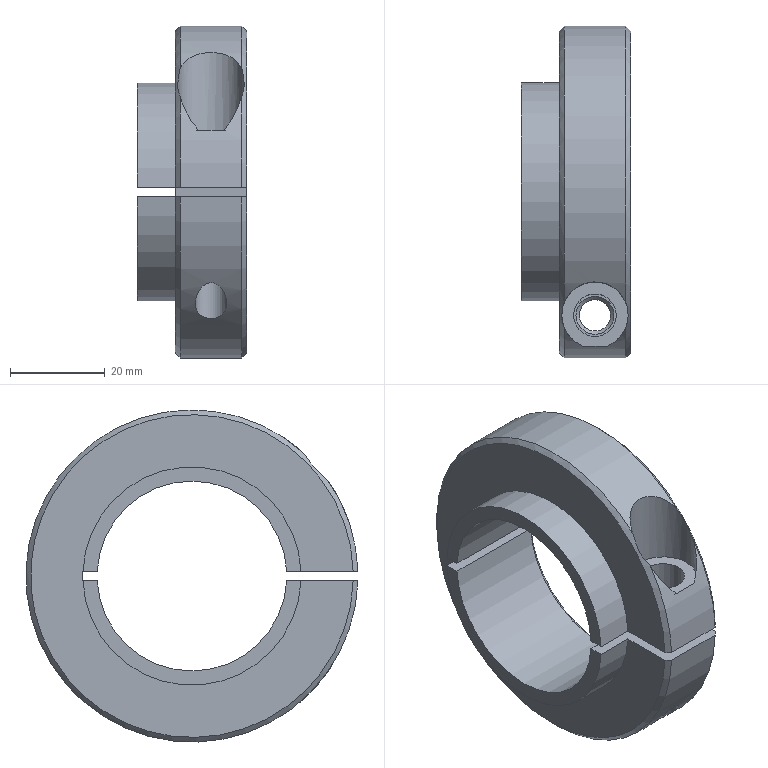Part | NX | features 1_52 2 | 1 solid | 24 faces | box 23 x 69.986 x 70 mm | volume 38156 mm3 | plane 10 | cylinder 9 | cone 5 | commonest cylinder face diameters 40 x2 46 x2 70 x2 6.647 x1 9 x1 14 x1
STEP:
#1=CARTESIAN_POINT('',(-138.5,-99.025,-821.129));
#2=VERTEX_POINT('',#1);
#3=CARTESIAN_POINT('',(-138.5,-138.975,-821.129));
#4=VERTEX_POINT('',#3);
#5=CARTESIAN_POINT('',(-138.5,-119.,-820.129));
#6=DIRECTION('',(-1.,0.,0.));
#7=DIRECTION('',(0.,0.,-1.));
#8=AXIS2_PLACEMENT_3D('',#5,#6,#7);
#9=CIRCLE('',#8,20.);
#10=EDGE_CURVE('',#2,#4,#9,.T.);
#11=ORIENTED_EDGE('',*,*,#10,.T.);
#12=CARTESIAN_POINT('',(-137.5,-139.976,-821.129));
#13=VERTEX_POINT('',#12);
#14=CARTESIAN_POINT('',(-137.5,-139.976,-821.129));
#15=CARTESIAN_POINT('',(-137.833,-139.642,-821.129));
#16=CARTESIAN_POINT('',(-138.167,-139.309,-821.129));
#17=CARTESIAN_POINT('',(-138.5,-138.975,-821.129));
#18=B_SPLINE_CURVE_WITH_KNOTS('',3,(#14,#15,#16,#17),.UNSPECIFIED.,.F.,.F.,(4,4),(0.,1.),.UNSPECIFIED.);
#19=EDGE_CURVE('',#4,#13,#18,.F.);
#20=ORIENTED_EDGE('',*,*,#19,.T.);
#21=CARTESIAN_POINT('',(-137.5,-98.024,-821.129));
#22=VERTEX_POINT('',#21);
#23=CARTESIAN_POINT('',(-137.5,-119.,-820.129));
#24=DIRECTION('',(-1.,0.,0.));
#25=DIRECTION('',(0.,0.,-1.));
#26=AXIS2_PLACEMENT_3D('',#23,#24,#25);
#27=CIRCLE('',#26,21.);
#28=EDGE_CURVE('',#22,#13,#27,.T.);
#29=ORIENTED_EDGE('',*,*,#28,.F.);
#30=CARTESIAN_POINT('',(-138.5,-99.025,-821.129));
#31=CARTESIAN_POINT('',(-138.167,-98.691,-821.129));
#32=CARTESIAN_POINT('',(-137.833,-98.358,-821.129));
#33=CARTESIAN_POINT('',(-137.5,-98.024,-821.129));
#34=B_SPLINE_CURVE_WITH_KNOTS('',3,(#30,#31,#32,#33),.UNSPECIFIED.,.F.,.F.,(4,4),(0.,1.),.UNSPECIFIED.);
#35=EDGE_CURVE('',#22,#2,#34,.F.);
#36=ORIENTED_EDGE('',*,*,#35,.T.);
#37=EDGE_LOOP('',(#11,#20,#29,#36));
#38=FACE_BOUND('',#37,.T.);
#39=CARTESIAN_POINT('',(-138.586,-119.,-820.129));
#40=DIRECTION('',(1.,0.,0.));
#41=DIRECTION('',(0.,0.,-1.));
#42=AXIS2_PLACEMENT_3D('',#39,#40,#41);
#43=CONICAL_SURFACE('',#42,19.914,0.7854);
#44=ADVANCED_FACE('',(#38),#43,.F.);
#45=CARTESIAN_POINT('',(-149.5,-145.,-819.129));
#46=VERTEX_POINT('',#45);
#47=CARTESIAN_POINT('',(-145.,-145.,-819.129));
#48=DIRECTION('',(0.,0.,1.));
#49=DIRECTION('',(-1.,0.,0.));
#50=AXIS2_PLACEMENT_3D('',#47,#48,#49);
#51=CIRCLE('',#50,4.5);
#52=EDGE_CURVE('',#46,#46,#51,.T.);
#53=ORIENTED_EDGE('',*,*,#52,.F.);
#54=EDGE_LOOP('',(#53));
#55=FACE_BOUND('',#54,.T.);
#56=CARTESIAN_POINT('',(-140.5,-145.,-807.129));
#57=VERTEX_POINT('',#56);
#58=CARTESIAN_POINT('',(-145.,-145.,-807.129));
#59=DIRECTION('',(0.,0.,-1.));
#60=DIRECTION('',(1.,0.,0.));
#61=AXIS2_PLACEMENT_3D('',#58,#59,#60);
#62=CIRCLE('',#61,4.5);
#63=EDGE_CURVE('',#57,#57,#62,.T.);
#64=ORIENTED_EDGE('',*,*,#63,.F.);
#65=EDGE_LOOP('',(#64));
#66=FACE_BOUND('',#65,.T.);
#67=CARTESIAN_POINT('',(-145.,-145.,-813.629));
#68=DIRECTION('',(0.,0.,1.));
#69=DIRECTION('',(1.,0.,0.));
#70=AXIS2_PLACEMENT_3D('',#67,#68,#69);
#71=CYLINDRICAL_SURFACE('',#70,4.5);
#72=ADVANCED_FACE('',(#55,#66),#71,.F.);
#73=CARTESIAN_POINT('',(-141.677,-145.,-821.806));
#74=VERTEX_POINT('',#73);
#75=CARTESIAN_POINT('',(-145.,-145.,-821.806));
#76=DIRECTION('',(0.,0.,-1.));
#77=DIRECTION('',(1.,0.,0.));
#78=AXIS2_PLACEMENT_3D('',#75,#76,#77);
#79=CIRCLE('',#78,3.323);
#80=EDGE_CURVE('',#74,#74,#79,.T.);
#81=ORIENTED_EDGE('',*,*,#80,.T.);
#82=EDGE_LOOP('',(#81));
#83=FACE_BOUND('',#82,.T.);
#84=CARTESIAN_POINT('',(-149.,-145.,-821.129));
#85=VERTEX_POINT('',#84);
#86=CARTESIAN_POINT('',(-145.,-145.,-821.129));
#87=DIRECTION('',(0.,0.,-1.));
#88=DIRECTION('',(-1.,0.,0.));
#89=AXIS2_PLACEMENT_3D('',#86,#87,#88);
#90=CIRCLE('',#89,4.);
#91=EDGE_CURVE('',#85,#85,#90,.T.);
#92=ORIENTED_EDGE('',*,*,#91,.F.);
#93=EDGE_LOOP('',(#92));
#94=FACE_BOUND('',#93,.T.);
#95=CARTESIAN_POINT('',(-145.,-145.,-821.892));
#96=DIRECTION('',(0.,0.,1.));
#97=DIRECTION('',(1.,0.,0.));
#98=AXIS2_PLACEMENT_3D('',#95,#96,#97);
#99=CONICAL_SURFACE('',#98,3.237,0.7854);
#100=ADVANCED_FACE('',(#83,#94),#99,.F.);
#101=CARTESIAN_POINT('',(-141.677,-145.,-843.56));
#102=VERTEX_POINT('',#101);
#103=CARTESIAN_POINT('',(-148.323,-145.,-843.56));
#104=VERTEX_POINT('',#103);
#105=CARTESIAN_POINT('',(-148.323,-145.,-843.56));
#106=CARTESIAN_POINT('',(-148.323,-145.388,-843.13));
#107=CARTESIAN_POINT('',(-148.191,-146.141,-842.25));
#108=CARTESIAN_POINT('',(-147.617,-147.152,-840.945));
#109=CARTESIAN_POINT('',(-146.673,-147.999,-839.739));
#110=CARTESIAN_POINT('',(-145.,-148.486,-838.987));
#111=CARTESIAN_POINT('',(-143.327,-147.999,-839.739));
#112=CARTESIAN_POINT('',(-142.383,-147.152,-840.945));
#113=CARTESIAN_POINT('',(-141.809,-146.141,-842.25));
#114=CARTESIAN_POINT('',(-141.677,-145.388,-843.13));
#115=CARTESIAN_POINT('',(-141.677,-145.,-843.56));
#116=B_SPLINE_CURVE_WITH_KNOTS('',3,(#105,#106,#107,#108,#109,#110,#111,#112,#113,#114,#115),.UNSPECIFIED.,.F.,.F.,(4,1,1,1,1,1,1,1,4),(0.,0.125,0.25,0.375,0.5,0.625,0.75,0.875,1.),.UNSPECIFIED.);
#117=EDGE_CURVE('',#102,#104,#116,.F.);
#118=ORIENTED_EDGE('',*,*,#117,.T.);
#119=CARTESIAN_POINT('',(-141.677,-145.,-843.56));
#120=CARTESIAN_POINT('',(-141.677,-144.295,-844.34));
#121=CARTESIAN_POINT('',(-142.002,-143.157,-845.485));
#122=CARTESIAN_POINT('',(-143.428,-141.943,-846.565));
#123=CARTESIAN_POINT('',(-145.,-141.543,-846.902));
#124=CARTESIAN_POINT('',(-146.572,-141.943,-846.565));
#125=CARTESIAN_POINT('',(-147.998,-143.157,-845.486));
#126=CARTESIAN_POINT('',(-148.323,-144.295,-844.34));
#127=CARTESIAN_POINT('',(-148.323,-145.,-843.56));
#128=B_SPLINE_CURVE_WITH_KNOTS('',3,(#119,#120,#121,#122,#123,#124,#125,#126,#127),.UNSPECIFIED.,.F.,.F.,(4,1,1,1,1,1,4),(0.,0.25,0.375,0.5,0.625,0.75,1.),.UNSPECIFIED.);
#129=EDGE_CURVE('',#104,#102,#128,.F.);
#130=ORIENTED_EDGE('',*,*,#129,.T.);
#131=EDGE_LOOP('',(#118,#130));
#132=FACE_BOUND('',#131,.T.);
#133=ORIENTED_EDGE('',*,*,#80,.F.);
#134=EDGE_LOOP('',(#133));
#135=FACE_BOUND('',#134,.T.);
#136=CARTESIAN_POINT('',(-145.,-145.,-840.968));
#137=DIRECTION('',(0.,0.,-1.));
#138=DIRECTION('',(-1.,0.,0.));
#139=AXIS2_PLACEMENT_3D('',#136,#137,#138);
#140=CYLINDRICAL_SURFACE('',#139,3.324);
#141=ADVANCED_FACE('',(#132,#135),#140,.F.);
#142=CARTESIAN_POINT('',(-151.5,-142.402,-794.103));
#143=VERTEX_POINT('',#142);
#144=CARTESIAN_POINT('',(-151.5,-153.986,-821.129));
#145=VERTEX_POINT('',#144);
#146=CARTESIAN_POINT('',(-151.5,-119.,-820.129));
#147=DIRECTION('',(-1.,0.,0.));
#148=DIRECTION('',(0.,-0.6686,0.7436));
#149=AXIS2_PLACEMENT_3D('',#146,#147,#148);
#150=CIRCLE('',#149,35.);
#151=EDGE_CURVE('',#143,#145,#150,.T.);
#152=ORIENTED_EDGE('',*,*,#151,.F.);
#153=CARTESIAN_POINT('',(-138.5,-142.402,-794.103));
#154=VERTEX_POINT('',#153);
#155=CARTESIAN_POINT('',(-138.5,-142.402,-794.103));
#156=CARTESIAN_POINT('',(-138.933,-141.315,-793.126));
#157=CARTESIAN_POINT('',(-140.459,-139.092,-791.412));
#158=CARTESIAN_POINT('',(-145.,-137.454,-790.398));
#159=CARTESIAN_POINT('',(-149.541,-139.092,-791.412));
#160=CARTESIAN_POINT('',(-151.068,-141.315,-793.126));
#161=CARTESIAN_POINT('',(-151.5,-142.402,-794.103));
#162=B_SPLINE_CURVE_WITH_KNOTS('',3,(#155,#156,#157,#158,#159,#160,#161),.UNSPECIFIED.,.F.,.F.,(4,1,1,1,4),(0.,0.25,0.5,0.75,1.),.UNSPECIFIED.);
#163=EDGE_CURVE('',#154,#143,#162,.T.);
#164=ORIENTED_EDGE('',*,*,#163,.F.);
#165=CARTESIAN_POINT('',(-138.5,-153.986,-821.129));
#166=VERTEX_POINT('',#165);
#167=CARTESIAN_POINT('',(-138.5,-119.,-820.129));
#168=DIRECTION('',(1.,0.,0.));
#169=DIRECTION('',(0.,0.,1.));
#170=AXIS2_PLACEMENT_3D('',#167,#168,#169);
#171=CIRCLE('',#170,35.);
#172=EDGE_CURVE('',#166,#154,#171,.T.);
#173=ORIENTED_EDGE('',*,*,#172,.F.);
#174=CARTESIAN_POINT('',(-138.5,-153.986,-821.129));
#175=DIRECTION('',(-1.,0.,0.));
#176=VECTOR('',#175,1000.);
#177=LINE('',#174,#176);
#178=EDGE_CURVE('',#166,#145,#177,.T.);
#179=ORIENTED_EDGE('',*,*,#178,.T.);
#180=EDGE_LOOP('',(#152,#164,#173,#179));
#181=FACE_BOUND('',#180,.T.);
#182=ORIENTED_EDGE('',*,*,#129,.F.);
#183=ORIENTED_EDGE('',*,*,#117,.F.);
#184=EDGE_LOOP('',(#182,#183));
#185=FACE_BOUND('',#184,.T.);
#186=CARTESIAN_POINT('',(-145.,-119.,-820.129));
#187=DIRECTION('',(1.,0.,0.));
#188=DIRECTION('',(0.,0.,-1.));
#189=AXIS2_PLACEMENT_3D('',#186,#187,#188);
#190=CYLINDRICAL_SURFACE('',#189,35.);
#191=ADVANCED_FACE('',(#181,#185),#190,.T.);
#192=ORIENTED_EDGE('',*,*,#63,.T.);
#193=EDGE_LOOP('',(#192));
#194=FACE_BOUND('',#193,.T.);
#195=CARTESIAN_POINT('',(-142.392,-151.496,-807.129));
#196=VERTEX_POINT('',#195);
#197=CARTESIAN_POINT('',(-147.608,-151.496,-807.129));
#198=VERTEX_POINT('',#197);
#199=CARTESIAN_POINT('',(-142.392,-151.496,-807.129));
#200=DIRECTION('',(-1.,0.,0.));
#201=VECTOR('',#200,1000.);
#202=LINE('',#199,#201);
#203=EDGE_CURVE('',#196,#198,#202,.T.);
#204=ORIENTED_EDGE('',*,*,#203,.F.);
#205=CARTESIAN_POINT('',(-145.,-145.,-807.129));
#206=DIRECTION('',(0.,0.,1.));
#207=DIRECTION('',(-1.,0.,0.));
#208=AXIS2_PLACEMENT_3D('',#205,#206,#207);
#209=CIRCLE('',#208,7.);
#210=EDGE_CURVE('',#196,#198,#209,.T.);
#211=ORIENTED_EDGE('',*,*,#210,.T.);
#212=EDGE_LOOP('',(#204,#211));
#213=FACE_BOUND('',#212,.T.);
#214=CARTESIAN_POINT('',(-145.,-150.75,-807.129));
#215=DIRECTION('',(0.,0.,-1.));
#216=DIRECTION('',(-1.,0.,0.));
#217=AXIS2_PLACEMENT_3D('',#214,#215,#216);
#218=PLANE('',#217);
#219=ADVANCED_FACE('',(#194,#213),#218,.F.);
#220=ORIENTED_EDGE('',*,*,#210,.F.);
#221=CARTESIAN_POINT('',(-138.5,-147.598,-799.951));
#222=VERTEX_POINT('',#221);
#223=CARTESIAN_POINT('',(-138.5,-147.598,-799.951));
#224=CARTESIAN_POINT('',(-138.843,-148.455,-801.166));
#225=CARTESIAN_POINT('',(-139.839,-149.967,-803.636));
#226=CARTESIAN_POINT('',(-141.357,-151.081,-806.087));
#227=CARTESIAN_POINT('',(-142.392,-151.496,-807.129));
#228=B_SPLINE_CURVE_WITH_KNOTS('',3,(#223,#224,#225,#226,#227),.UNSPECIFIED.,.F.,.F.,(4,1,4),(0.,0.5,1.),.UNSPECIFIED.);
#229=EDGE_CURVE('',#196,#222,#228,.F.);
#230=ORIENTED_EDGE('',*,*,#229,.T.);
#231=CARTESIAN_POINT('',(-138.,-145.,-797.452));
#232=VERTEX_POINT('',#231);
#233=CARTESIAN_POINT('',(-138.,-145.,-797.452));
#234=CARTESIAN_POINT('',(-138.,-145.806,-798.364));
#235=CARTESIAN_POINT('',(-138.124,-146.657,-799.264));
#236=CARTESIAN_POINT('',(-138.5,-147.598,-799.951));
#237=B_SPLINE_CURVE_WITH_KNOTS('',3,(#233,#234,#235,#236),.UNSPECIFIED.,.F.,.F.,(4,4),(0.,1.),.UNSPECIFIED.);
#238=EDGE_CURVE('',#222,#232,#237,.F.);
#239=ORIENTED_EDGE('',*,*,#238,.T.);
#240=CARTESIAN_POINT('',(-138.5,-142.402,-794.103));
#241=CARTESIAN_POINT('',(-138.182,-143.198,-795.243));
#242=CARTESIAN_POINT('',(-138.,-144.063,-796.376));
#243=CARTESIAN_POINT('',(-138.,-145.,-797.452));
#244=B_SPLINE_CURVE_WITH_KNOTS('',3,(#240,#241,#242,#243),.UNSPECIFIED.,.F.,.F.,(4,4),(0.,1.),.UNSPECIFIED.);
#245=EDGE_CURVE('',#232,#154,#244,.F.);
#246=ORIENTED_EDGE('',*,*,#245,.T.);
#247=ORIENTED_EDGE('',*,*,#163,.T.);
#248=CARTESIAN_POINT('',(-152.,-145.,-797.452));
#249=VERTEX_POINT('',#248);
#250=CARTESIAN_POINT('',(-152.,-145.,-797.452));
#251=CARTESIAN_POINT('',(-152.,-144.063,-796.376));
#252=CARTESIAN_POINT('',(-151.818,-143.198,-795.243));
#253=CARTESIAN_POINT('',(-151.5,-142.402,-794.103));
#254=B_SPLINE_CURVE_WITH_KNOTS('',3,(#250,#251,#252,#253),.UNSPECIFIED.,.F.,.F.,(4,4),(0.,1.),.UNSPECIFIED.);
#255=EDGE_CURVE('',#143,#249,#254,.F.);
#256=ORIENTED_EDGE('',*,*,#255,.T.);
#257=CARTESIAN_POINT('',(-151.5,-147.598,-799.951));
#258=VERTEX_POINT('',#257);
#259=CARTESIAN_POINT('',(-151.5,-147.598,-799.951));
#260=CARTESIAN_POINT('',(-151.876,-146.657,-799.264));
#261=CARTESIAN_POINT('',(-152.,-145.806,-798.363));
#262=CARTESIAN_POINT('',(-152.,-145.,-797.452));
#263=B_SPLINE_CURVE_WITH_KNOTS('',3,(#259,#260,#261,#262),.UNSPECIFIED.,.F.,.F.,(4,4),(0.,1.),.UNSPECIFIED.);
#264=EDGE_CURVE('',#249,#258,#263,.F.);
#265=ORIENTED_EDGE('',*,*,#264,.T.);
#266=CARTESIAN_POINT('',(-147.608,-151.496,-807.129));
#267=CARTESIAN_POINT('',(-148.643,-151.081,-806.087));
#268=CARTESIAN_POINT('',(-150.161,-149.967,-803.636));
#269=CARTESIAN_POINT('',(-151.157,-148.455,-801.166));
#270=CARTESIAN_POINT('',(-151.5,-147.598,-799.951));
#271=B_SPLINE_CURVE_WITH_KNOTS('',3,(#266,#267,#268,#269,#270),.UNSPECIFIED.,.F.,.F.,(4,1,4),(0.,0.5,1.),.UNSPECIFIED.);
#272=EDGE_CURVE('',#258,#198,#271,.F.);
#273=ORIENTED_EDGE('',*,*,#272,.T.);
#274=EDGE_LOOP('',(#220,#230,#239,#246,#247,#256,#265,#273));
#275=FACE_BOUND('',#274,.T.);
#276=CARTESIAN_POINT('',(-145.,-145.,-796.129));
#277=DIRECTION('',(0.,0.,1.));
#278=DIRECTION('',(1.,0.,0.));
#279=AXIS2_PLACEMENT_3D('',#276,#277,#278);
#280=CYLINDRICAL_SURFACE('',#279,7.);
#281=ADVANCED_FACE('',(#275),#280,.F.);
#282=CARTESIAN_POINT('',(-138.5,-153.986,-819.129));
#283=VERTEX_POINT('',#282);
#284=CARTESIAN_POINT('',(-138.5,-119.,-820.129));
#285=DIRECTION('',(1.,0.,0.));
#286=DIRECTION('',(0.,-0.8171,0.5765));
#287=AXIS2_PLACEMENT_3D('',#284,#285,#286);
#288=CIRCLE('',#287,35.);
#289=EDGE_CURVE('',#222,#283,#288,.T.);
#290=ORIENTED_EDGE('',*,*,#289,.F.);
#291=ORIENTED_EDGE('',*,*,#229,.F.);
#292=ORIENTED_EDGE('',*,*,#203,.T.);
#293=ORIENTED_EDGE('',*,*,#272,.F.);
#294=CARTESIAN_POINT('',(-151.5,-153.986,-819.129));
#295=VERTEX_POINT('',#294);
#296=CARTESIAN_POINT('',(-151.5,-119.,-820.129));
#297=DIRECTION('',(-1.,0.,0.));
#298=DIRECTION('',(0.,-0.9996,0.02857));
#299=AXIS2_PLACEMENT_3D('',#296,#297,#298);
#300=CIRCLE('',#299,35.);
#301=EDGE_CURVE('',#295,#258,#300,.T.);
#302=ORIENTED_EDGE('',*,*,#301,.F.);
#303=CARTESIAN_POINT('',(-151.5,-153.986,-819.129));
#304=DIRECTION('',(1.,0.,0.));
#305=VECTOR('',#304,1000.);
#306=LINE('',#303,#305);
#307=EDGE_CURVE('',#295,#283,#306,.T.);
#308=ORIENTED_EDGE('',*,*,#307,.T.);
#309=EDGE_LOOP('',(#290,#291,#292,#293,#302,#308));
#310=FACE_BOUND('',#309,.T.);
#311=CARTESIAN_POINT('',(-145.,-119.,-820.129));
#312=DIRECTION('',(1.,0.,0.));
#313=DIRECTION('',(0.,0.,-1.));
#314=AXIS2_PLACEMENT_3D('',#311,#312,#313);
#315=CYLINDRICAL_SURFACE('',#314,35.);
#316=ADVANCED_FACE('',(#310),#315,.T.);
#317=CARTESIAN_POINT('',(-137.5,-152.985,-821.129));
#318=VERTEX_POINT('',#317);
#319=CARTESIAN_POINT('',(-137.5,-152.985,-819.129));
#320=VERTEX_POINT('',#319);
#321=CARTESIAN_POINT('',(-137.5,-119.,-820.129));
#322=DIRECTION('',(1.,0.,0.));
#323=DIRECTION('',(0.,0.,1.));
#324=AXIS2_PLACEMENT_3D('',#321,#322,#323);
#325=CIRCLE('',#324,34.);
#326=EDGE_CURVE('',#318,#320,#325,.T.);
#327=ORIENTED_EDGE('',*,*,#326,.F.);
#328=CARTESIAN_POINT('',(-138.5,-153.986,-821.129));
#329=CARTESIAN_POINT('',(-138.167,-153.652,-821.129));
#330=CARTESIAN_POINT('',(-137.833,-153.319,-821.129));
#331=CARTESIAN_POINT('',(-137.5,-152.985,-821.129));
#332=B_SPLINE_CURVE_WITH_KNOTS('',3,(#328,#329,#330,#331),.UNSPECIFIED.,.F.,.F.,(4,4),(0.,1.),.UNSPECIFIED.);
#333=EDGE_CURVE('',#318,#166,#332,.F.);
#334=ORIENTED_EDGE('',*,*,#333,.T.);
#335=ORIENTED_EDGE('',*,*,#172,.T.);
#336=ORIENTED_EDGE('',*,*,#245,.F.);
#337=ORIENTED_EDGE('',*,*,#238,.F.);
#338=ORIENTED_EDGE('',*,*,#289,.T.);
#339=CARTESIAN_POINT('',(-137.5,-152.985,-819.129));
#340=CARTESIAN_POINT('',(-137.833,-153.319,-819.129));
#341=CARTESIAN_POINT('',(-138.167,-153.652,-819.129));
#342=CARTESIAN_POINT('',(-138.5,-153.986,-819.129));
#343=B_SPLINE_CURVE_WITH_KNOTS('',3,(#339,#340,#341,#342),.UNSPECIFIED.,.F.,.F.,(4,4),(0.,1.),.UNSPECIFIED.);
#344=EDGE_CURVE('',#283,#320,#343,.F.);
#345=ORIENTED_EDGE('',*,*,#344,.T.);
#346=EDGE_LOOP('',(#327,#334,#335,#336,#337,#338,#345));
#347=FACE_BOUND('',#346,.T.);
#348=CARTESIAN_POINT('',(-137.414,-119.,-820.129));
#349=DIRECTION('',(-1.,0.,0.));
#350=DIRECTION('',(0.,0.,1.));
#351=AXIS2_PLACEMENT_3D('',#348,#349,#350);
#352=CONICAL_SURFACE('',#351,33.914,0.7854);
#353=ADVANCED_FACE('',(#347),#352,.T.);
#354=CARTESIAN_POINT('',(-160.5,-99.025,-819.129));
#355=VERTEX_POINT('',#354);
#356=CARTESIAN_POINT('',(-138.5,-99.025,-819.129));
#357=VERTEX_POINT('',#356);
#358=CARTESIAN_POINT('',(-160.5,-99.025,-819.129));
#359=DIRECTION('',(1.,0.,0.));
#360=VECTOR('',#359,1000.);
#361=LINE('',#358,#360);
#362=EDGE_CURVE('',#355,#357,#361,.T.);
#363=ORIENTED_EDGE('',*,*,#362,.T.);
#364=CARTESIAN_POINT('',(-138.5,-138.975,-819.129));
#365=VERTEX_POINT('',#364);
#366=CARTESIAN_POINT('',(-138.5,-119.,-820.129));
#367=DIRECTION('',(-1.,0.,0.));
#368=DIRECTION('',(0.,0.,1.));
#369=AXIS2_PLACEMENT_3D('',#366,#367,#368);
#370=CIRCLE('',#369,20.);
#371=EDGE_CURVE('',#365,#357,#370,.T.);
#372=ORIENTED_EDGE('',*,*,#371,.F.);
#373=CARTESIAN_POINT('',(-160.5,-138.975,-819.129));
#374=VERTEX_POINT('',#373);
#375=CARTESIAN_POINT('',(-138.5,-138.975,-819.129));
#376=DIRECTION('',(-1.,0.,0.));
#377=VECTOR('',#376,1000.);
#378=LINE('',#375,#377);
#379=EDGE_CURVE('',#365,#374,#378,.T.);
#380=ORIENTED_EDGE('',*,*,#379,.T.);
#381=CARTESIAN_POINT('',(-160.5,-119.,-820.129));
#382=DIRECTION('',(1.,0.,0.));
#383=DIRECTION('',(0.,0.9987,0.05));
#384=AXIS2_PLACEMENT_3D('',#381,#382,#383);
#385=CIRCLE('',#384,20.);
#386=EDGE_CURVE('',#355,#374,#385,.T.);
#387=ORIENTED_EDGE('',*,*,#386,.F.);
#388=EDGE_LOOP('',(#363,#372,#380,#387));
#389=FACE_BOUND('',#388,.T.);
#390=CARTESIAN_POINT('',(-160.5,-119.,-820.129));
#391=DIRECTION('',(1.,0.,0.));
#392=DIRECTION('',(0.,0.,-1.));
#393=AXIS2_PLACEMENT_3D('',#390,#391,#392);
#394=CYLINDRICAL_SURFACE('',#393,20.);
#395=ADVANCED_FACE('',(#389),#394,.F.);
#396=CARTESIAN_POINT('',(-137.5,-139.976,-819.129));
#397=VERTEX_POINT('',#396);
#398=CARTESIAN_POINT('',(-137.5,-98.024,-819.129));
#399=VERTEX_POINT('',#398);
#400=CARTESIAN_POINT('',(-137.5,-119.,-820.129));
#401=DIRECTION('',(-1.,0.,0.));
#402=DIRECTION('',(0.,0.,1.));
#403=AXIS2_PLACEMENT_3D('',#400,#401,#402);
#404=CIRCLE('',#403,21.);
#405=EDGE_CURVE('',#397,#399,#404,.T.);
#406=ORIENTED_EDGE('',*,*,#405,.F.);
#407=CARTESIAN_POINT('',(-138.5,-138.975,-819.129));
#408=CARTESIAN_POINT('',(-138.167,-139.309,-819.129));
#409=CARTESIAN_POINT('',(-137.833,-139.642,-819.129));
#410=CARTESIAN_POINT('',(-137.5,-139.976,-819.129));
#411=B_SPLINE_CURVE_WITH_KNOTS('',3,(#407,#408,#409,#410),.UNSPECIFIED.,.F.,.F.,(4,4),(0.,1.),.UNSPECIFIED.);
#412=EDGE_CURVE('',#397,#365,#411,.F.);
#413=ORIENTED_EDGE('',*,*,#412,.T.);
#414=ORIENTED_EDGE('',*,*,#371,.T.);
#415=CARTESIAN_POINT('',(-137.5,-98.024,-819.129));
#416=CARTESIAN_POINT('',(-137.833,-98.358,-819.129));
#417=CARTESIAN_POINT('',(-138.167,-98.691,-819.129));
#418=CARTESIAN_POINT('',(-138.5,-99.025,-819.129));
#419=B_SPLINE_CURVE_WITH_KNOTS('',3,(#415,#416,#417,#418),.UNSPECIFIED.,.F.,.F.,(4,4),(0.,1.),.UNSPECIFIED.);
#420=EDGE_CURVE('',#357,#399,#419,.F.);
#421=ORIENTED_EDGE('',*,*,#420,.T.);
#422=EDGE_LOOP('',(#406,#413,#414,#421));
#423=FACE_BOUND('',#422,.T.);
#424=CARTESIAN_POINT('',(-138.586,-119.,-820.129));
#425=DIRECTION('',(1.,0.,0.));
#426=DIRECTION('',(0.,0.,-1.));
#427=AXIS2_PLACEMENT_3D('',#424,#425,#426);
#428=CONICAL_SURFACE('',#427,19.914,0.7854);
#429=ADVANCED_FACE('',(#423),#428,.F.);
#430=CARTESIAN_POINT('',(-137.5,-96.,-821.129));
#431=VERTEX_POINT('',#430);
#432=CARTESIAN_POINT('',(-137.5,-98.024,-821.129));
#433=DIRECTION('',(0.,1.,0.));
#434=VECTOR('',#433,1000.);
#435=LINE('',#432,#434);
#436=EDGE_CURVE('',#22,#431,#435,.T.);
#437=ORIENTED_EDGE('',*,*,#436,.F.);
#438=ORIENTED_EDGE('',*,*,#28,.T.);
#439=CARTESIAN_POINT('',(-137.5,-152.985,-821.129));
#440=DIRECTION('',(0.,1.,0.));
#441=VECTOR('',#440,1000.);
#442=LINE('',#439,#441);
#443=EDGE_CURVE('',#318,#13,#442,.T.);
#444=ORIENTED_EDGE('',*,*,#443,.F.);
#445=ORIENTED_EDGE('',*,*,#326,.T.);
#446=CARTESIAN_POINT('',(-137.5,-139.976,-819.129));
#447=DIRECTION('',(0.,-1.,0.));
#448=VECTOR('',#447,1000.);
#449=LINE('',#446,#448);
#450=EDGE_CURVE('',#397,#320,#449,.T.);
#451=ORIENTED_EDGE('',*,*,#450,.F.);
#452=ORIENTED_EDGE('',*,*,#405,.T.);
#453=CARTESIAN_POINT('',(-137.5,-96.,-819.129));
#454=VERTEX_POINT('',#453);
#455=CARTESIAN_POINT('',(-137.5,-96.,-819.129));
#456=DIRECTION('',(0.,-1.,0.));
#457=VECTOR('',#456,1000.);
#458=LINE('',#455,#457);
#459=EDGE_CURVE('',#454,#399,#458,.T.);
#460=ORIENTED_EDGE('',*,*,#459,.F.);
#461=CARTESIAN_POINT('',(-137.5,-96.,-821.129));
#462=DIRECTION('',(0.,0.,1.));
#463=VECTOR('',#462,1000.);
#464=LINE('',#461,#463);
#465=EDGE_CURVE('',#431,#454,#464,.T.);
#466=ORIENTED_EDGE('',*,*,#465,.F.);
#467=EDGE_LOOP('',(#437,#438,#444,#445,#451,#452,#460,#466));
#468=FACE_BOUND('',#467,.T.);
#469=CARTESIAN_POINT('',(-137.5,-91.5,-820.129));
#470=DIRECTION('',(1.,0.,0.));
#471=DIRECTION('',(0.,0.,-1.));
#472=AXIS2_PLACEMENT_3D('',#469,#470,#471);
#473=PLANE('',#472);
#474=ADVANCED_FACE('',(#468),#473,.T.);
#475=ORIENTED_EDGE('',*,*,#465,.T.);
#476=CARTESIAN_POINT('',(-152.5,-96.,-819.129));
#477=VERTEX_POINT('',#476);
#478=CARTESIAN_POINT('',(-137.5,-96.,-819.129));
#479=DIRECTION('',(-1.,0.,0.));
#480=VECTOR('',#479,1000.);
#481=LINE('',#478,#480);
#482=EDGE_CURVE('',#454,#477,#481,.T.);
#483=ORIENTED_EDGE('',*,*,#482,.T.);
#484=CARTESIAN_POINT('',(-152.5,-96.,-821.129));
#485=VERTEX_POINT('',#484);
#486=CARTESIAN_POINT('',(-152.5,-96.,-819.129));
#487=DIRECTION('',(0.,0.,-1.));
#488=VECTOR('',#487,1000.);
#489=LINE('',#486,#488);
#490=EDGE_CURVE('',#477,#485,#489,.T.);
#491=ORIENTED_EDGE('',*,*,#490,.T.);
#492=CARTESIAN_POINT('',(-137.5,-96.,-821.129));
#493=DIRECTION('',(-1.,0.,0.));
#494=VECTOR('',#493,1000.);
#495=LINE('',#492,#494);
#496=EDGE_CURVE('',#431,#485,#495,.T.);
#497=ORIENTED_EDGE('',*,*,#496,.F.);
#498=EDGE_LOOP('',(#475,#483,#491,#497));
#499=FACE_BOUND('',#498,.T.);
#500=CARTESIAN_POINT('',(-115.,-96.,-821.129));
#501=DIRECTION('',(0.,1.,0.));
#502=DIRECTION('',(0.,0.,1.));
#503=AXIS2_PLACEMENT_3D('',#500,#501,#502);
#504=PLANE('',#503);
#505=ADVANCED_FACE('',(#499),#504,.F.);
#506=CARTESIAN_POINT('',(-160.5,-99.025,-821.129));
#507=VERTEX_POINT('',#506);
#508=CARTESIAN_POINT('',(-160.5,-96.022,-821.129));
#509=VERTEX_POINT('',#508);
#510=CARTESIAN_POINT('',(-160.5,-99.025,-821.129));
#511=DIRECTION('',(0.,1.,0.));
#512=VECTOR('',#511,1000.);
#513=LINE('',#510,#512);
#514=EDGE_CURVE('',#507,#509,#513,.T.);
#515=ORIENTED_EDGE('',*,*,#514,.F.);
#516=CARTESIAN_POINT('',(-138.5,-99.025,-821.129));
#517=DIRECTION('',(-1.,0.,0.));
#518=VECTOR('',#517,1000.);
#519=LINE('',#516,#518);
#520=EDGE_CURVE('',#2,#507,#519,.T.);
#521=ORIENTED_EDGE('',*,*,#520,.F.);
#522=ORIENTED_EDGE('',*,*,#35,.F.);
#523=ORIENTED_EDGE('',*,*,#436,.T.);
#524=ORIENTED_EDGE('',*,*,#496,.T.);
#525=CARTESIAN_POINT('',(-152.5,-96.022,-821.129));
#526=VERTEX_POINT('',#525);
#527=CARTESIAN_POINT('',(-152.5,-96.,-821.129));
#528=DIRECTION('',(0.,-1.,0.));
#529=VECTOR('',#528,1000.);
#530=LINE('',#527,#529);
#531=EDGE_CURVE('',#485,#526,#530,.T.);
#532=ORIENTED_EDGE('',*,*,#531,.T.);
#533=CARTESIAN_POINT('',(-160.5,-96.022,-821.129));
#534=DIRECTION('',(1.,0.,0.));
#535=VECTOR('',#534,1000.);
#536=LINE('',#533,#535);
#537=EDGE_CURVE('',#509,#526,#536,.T.);
#538=ORIENTED_EDGE('',*,*,#537,.F.);
#539=EDGE_LOOP('',(#515,#521,#522,#523,#524,#532,#538));
#540=FACE_BOUND('',#539,.T.);
#541=CARTESIAN_POINT('',(-160.5,-96.,-821.129));
#542=DIRECTION('',(0.,0.,1.));
#543=DIRECTION('',(1.,0.,0.));
#544=AXIS2_PLACEMENT_3D('',#541,#542,#543);
#545=PLANE('',#544);
#546=ADVANCED_FACE('',(#540),#545,.T.);
#547=CARTESIAN_POINT('',(-160.5,-138.975,-821.129));
#548=VERTEX_POINT('',#547);
#549=CARTESIAN_POINT('',(-160.5,-119.,-820.129));
#550=DIRECTION('',(1.,0.,0.));
#551=DIRECTION('',(0.,0.,-1.));
#552=AXIS2_PLACEMENT_3D('',#549,#550,#551);
#553=CIRCLE('',#552,20.);
#554=EDGE_CURVE('',#548,#507,#553,.T.);
#555=ORIENTED_EDGE('',*,*,#554,.F.);
#556=CARTESIAN_POINT('',(-160.5,-138.975,-821.129));
#557=DIRECTION('',(1.,0.,0.));
#558=VECTOR('',#557,1000.);
#559=LINE('',#556,#558);
#560=EDGE_CURVE('',#548,#4,#559,.T.);
#561=ORIENTED_EDGE('',*,*,#560,.T.);
#562=ORIENTED_EDGE('',*,*,#10,.F.);
#563=ORIENTED_EDGE('',*,*,#520,.T.);
#564=EDGE_LOOP('',(#555,#561,#562,#563));
#565=FACE_BOUND('',#564,.T.);
#566=CARTESIAN_POINT('',(-160.5,-119.,-820.129));
#567=DIRECTION('',(1.,0.,0.));
#568=DIRECTION('',(0.,0.,-1.));
#569=AXIS2_PLACEMENT_3D('',#566,#567,#568);
#570=CYLINDRICAL_SURFACE('',#569,20.);
#571=ADVANCED_FACE('',(#565),#570,.F.);
#572=ORIENTED_EDGE('',*,*,#91,.T.);
#573=EDGE_LOOP('',(#572));
#574=FACE_BOUND('',#573,.T.);
#575=CARTESIAN_POINT('',(-152.5,-141.978,-821.129));
#576=VERTEX_POINT('',#575);
#577=CARTESIAN_POINT('',(-152.5,-152.985,-821.129));
#578=VERTEX_POINT('',#577);
#579=CARTESIAN_POINT('',(-152.5,-141.978,-821.129));
#580=DIRECTION('',(0.,-1.,0.));
#581=VECTOR('',#580,1000.);
#582=LINE('',#579,#581);
#583=EDGE_CURVE('',#576,#578,#582,.T.);
#584=ORIENTED_EDGE('',*,*,#583,.T.);
#585=CARTESIAN_POINT('',(-152.5,-152.985,-821.129));
#586=CARTESIAN_POINT('',(-152.167,-153.319,-821.129));
#587=CARTESIAN_POINT('',(-151.833,-153.652,-821.129));
#588=CARTESIAN_POINT('',(-151.5,-153.986,-821.129));
#589=B_SPLINE_CURVE_WITH_KNOTS('',3,(#585,#586,#587,#588),.UNSPECIFIED.,.F.,.F.,(4,4),(0.,1.),.UNSPECIFIED.);
#590=EDGE_CURVE('',#145,#578,#589,.F.);
#591=ORIENTED_EDGE('',*,*,#590,.F.);
#592=ORIENTED_EDGE('',*,*,#178,.F.);
#593=ORIENTED_EDGE('',*,*,#333,.F.);
#594=ORIENTED_EDGE('',*,*,#443,.T.);
#595=ORIENTED_EDGE('',*,*,#19,.F.);
#596=ORIENTED_EDGE('',*,*,#560,.F.);
#597=CARTESIAN_POINT('',(-160.5,-141.978,-821.129));
#598=VERTEX_POINT('',#597);
#599=CARTESIAN_POINT('',(-160.5,-141.978,-821.129));
#600=DIRECTION('',(0.,1.,0.));
#601=VECTOR('',#600,1000.);
#602=LINE('',#599,#601);
#603=EDGE_CURVE('',#598,#548,#602,.T.);
#604=ORIENTED_EDGE('',*,*,#603,.F.);
#605=CARTESIAN_POINT('',(-152.5,-141.978,-821.129));
#606=DIRECTION('',(-1.,0.,0.));
#607=VECTOR('',#606,1000.);
#608=LINE('',#605,#607);
#609=EDGE_CURVE('',#576,#598,#608,.T.);
#610=ORIENTED_EDGE('',*,*,#609,.F.);
#611=EDGE_LOOP('',(#584,#591,#592,#593,#594,#595,#596,#604,#610));
#612=FACE_BOUND('',#611,.T.);
#613=CARTESIAN_POINT('',(-160.5,-96.,-821.129));
#614=DIRECTION('',(0.,0.,1.));
#615=DIRECTION('',(1.,0.,0.));
#616=AXIS2_PLACEMENT_3D('',#613,#614,#615);
#617=PLANE('',#616);
#618=ADVANCED_FACE('',(#574,#612),#617,.T.);
#619=CARTESIAN_POINT('',(-152.5,-152.985,-819.129));
#620=VERTEX_POINT('',#619);
#621=CARTESIAN_POINT('',(-152.5,-119.,-820.129));
#622=DIRECTION('',(-1.,0.,0.));
#623=DIRECTION('',(0.,0.,-1.));
#624=AXIS2_PLACEMENT_3D('',#621,#622,#623);
#625=CIRCLE('',#624,34.);
#626=EDGE_CURVE('',#620,#578,#625,.T.);
#627=ORIENTED_EDGE('',*,*,#626,.F.);
#628=CARTESIAN_POINT('',(-151.5,-153.986,-819.129));
#629=CARTESIAN_POINT('',(-151.833,-153.652,-819.129));
#630=CARTESIAN_POINT('',(-152.167,-153.319,-819.129));
#631=CARTESIAN_POINT('',(-152.5,-152.985,-819.129));
#632=B_SPLINE_CURVE_WITH_KNOTS('',3,(#628,#629,#630,#631),.UNSPECIFIED.,.F.,.F.,(4,4),(0.,1.),.UNSPECIFIED.);
#633=EDGE_CURVE('',#620,#295,#632,.F.);
#634=ORIENTED_EDGE('',*,*,#633,.T.);
#635=ORIENTED_EDGE('',*,*,#301,.T.);
#636=ORIENTED_EDGE('',*,*,#264,.F.);
#637=ORIENTED_EDGE('',*,*,#255,.F.);
#638=ORIENTED_EDGE('',*,*,#151,.T.);
#639=ORIENTED_EDGE('',*,*,#590,.T.);
#640=EDGE_LOOP('',(#627,#634,#635,#636,#637,#638,#639));
#641=FACE_BOUND('',#640,.T.);
#642=CARTESIAN_POINT('',(-152.586,-119.,-820.129));
#643=DIRECTION('',(1.,0.,0.));
#644=DIRECTION('',(0.,0.,-1.));
#645=AXIS2_PLACEMENT_3D('',#642,#643,#644);
#646=CONICAL_SURFACE('',#645,33.914,0.7854);
#647=ADVANCED_FACE('',(#641),#646,.T.);
#648=ORIENTED_EDGE('',*,*,#52,.T.);
#649=EDGE_LOOP('',(#648));
#650=FACE_BOUND('',#649,.T.);
#651=CARTESIAN_POINT('',(-160.5,-141.978,-819.129));
#652=VERTEX_POINT('',#651);
#653=CARTESIAN_POINT('',(-160.5,-138.975,-819.129));
#654=DIRECTION('',(0.,-1.,0.));
#655=VECTOR('',#654,1000.);
#656=LINE('',#653,#655);
#657=EDGE_CURVE('',#374,#652,#656,.T.);
#658=ORIENTED_EDGE('',*,*,#657,.F.);
#659=ORIENTED_EDGE('',*,*,#379,.F.);
#660=ORIENTED_EDGE('',*,*,#412,.F.);
#661=ORIENTED_EDGE('',*,*,#450,.T.);
#662=ORIENTED_EDGE('',*,*,#344,.F.);
#663=ORIENTED_EDGE('',*,*,#307,.F.);
#664=ORIENTED_EDGE('',*,*,#633,.F.);
#665=CARTESIAN_POINT('',(-152.5,-141.978,-819.129));
#666=VERTEX_POINT('',#665);
#667=CARTESIAN_POINT('',(-152.5,-152.985,-819.129));
#668=DIRECTION('',(0.,1.,0.));
#669=VECTOR('',#668,1000.);
#670=LINE('',#667,#669);
#671=EDGE_CURVE('',#620,#666,#670,.T.);
#672=ORIENTED_EDGE('',*,*,#671,.T.);
#673=CARTESIAN_POINT('',(-160.5,-141.978,-819.129));
#674=DIRECTION('',(1.,0.,0.));
#675=VECTOR('',#674,1000.);
#676=LINE('',#673,#675);
#677=EDGE_CURVE('',#652,#666,#676,.T.);
#678=ORIENTED_EDGE('',*,*,#677,.F.);
#679=EDGE_LOOP('',(#658,#659,#660,#661,#662,#663,#664,#672,#678));
#680=FACE_BOUND('',#679,.T.);
#681=CARTESIAN_POINT('',(-160.5,-96.,-819.129));
#682=DIRECTION('',(0.,0.,-1.));
#683=DIRECTION('',(-1.,0.,0.));
#684=AXIS2_PLACEMENT_3D('',#681,#682,#683);
#685=PLANE('',#684);
#686=ADVANCED_FACE('',(#650,#680),#685,.T.);
#687=CARTESIAN_POINT('',(-160.5,-96.022,-819.129));
#688=VERTEX_POINT('',#687);
#689=CARTESIAN_POINT('',(-160.5,-96.022,-819.129));
#690=DIRECTION('',(0.,-1.,0.));
#691=VECTOR('',#690,1000.);
#692=LINE('',#689,#691);
#693=EDGE_CURVE('',#688,#355,#692,.T.);
#694=ORIENTED_EDGE('',*,*,#693,.T.);
#695=ORIENTED_EDGE('',*,*,#386,.T.);
#696=ORIENTED_EDGE('',*,*,#657,.T.);
#697=CARTESIAN_POINT('',(-160.5,-119.,-820.129));
#698=DIRECTION('',(-1.,0.,0.));
#699=DIRECTION('',(0.,-0.9991,0.04348));
#700=AXIS2_PLACEMENT_3D('',#697,#698,#699);
#701=CIRCLE('',#700,23.);
#702=EDGE_CURVE('',#652,#688,#701,.T.);
#703=ORIENTED_EDGE('',*,*,#702,.T.);
#704=EDGE_LOOP('',(#694,#695,#696,#703));
#705=FACE_BOUND('',#704,.T.);
#706=CARTESIAN_POINT('',(-160.5,-119.,-820.129));
#707=DIRECTION('',(-1.,0.,0.));
#708=DIRECTION('',(0.,0.,1.));
#709=AXIS2_PLACEMENT_3D('',#706,#707,#708);
#710=PLANE('',#709);
#711=ADVANCED_FACE('',(#705),#710,.T.);
#712=CARTESIAN_POINT('',(-152.5,-96.022,-819.129));
#713=VERTEX_POINT('',#712);
#714=CARTESIAN_POINT('',(-152.5,-96.022,-819.129));
#715=DIRECTION('',(0.,1.,0.));
#716=VECTOR('',#715,1000.);
#717=LINE('',#714,#716);
#718=EDGE_CURVE('',#713,#477,#717,.T.);
#719=ORIENTED_EDGE('',*,*,#718,.T.);
#720=ORIENTED_EDGE('',*,*,#482,.F.);
#721=ORIENTED_EDGE('',*,*,#459,.T.);
#722=ORIENTED_EDGE('',*,*,#420,.F.);
#723=ORIENTED_EDGE('',*,*,#362,.F.);
#724=ORIENTED_EDGE('',*,*,#693,.F.);
#725=CARTESIAN_POINT('',(-152.5,-96.022,-819.129));
#726=DIRECTION('',(-1.,0.,0.));
#727=VECTOR('',#726,1000.);
#728=LINE('',#725,#727);
#729=EDGE_CURVE('',#713,#688,#728,.T.);
#730=ORIENTED_EDGE('',*,*,#729,.F.);
#731=EDGE_LOOP('',(#719,#720,#721,#722,#723,#724,#730));
#732=FACE_BOUND('',#731,.T.);
#733=CARTESIAN_POINT('',(-160.5,-96.,-819.129));
#734=DIRECTION('',(0.,0.,-1.));
#735=DIRECTION('',(-1.,0.,0.));
#736=AXIS2_PLACEMENT_3D('',#733,#734,#735);
#737=PLANE('',#736);
#738=ADVANCED_FACE('',(#732),#737,.T.);
#739=ORIENTED_EDGE('',*,*,#702,.F.);
#740=ORIENTED_EDGE('',*,*,#677,.T.);
#741=CARTESIAN_POINT('',(-152.5,-119.,-820.129));
#742=DIRECTION('',(1.,0.,0.));
#743=DIRECTION('',(0.,0.9991,0.04348));
#744=AXIS2_PLACEMENT_3D('',#741,#742,#743);
#745=CIRCLE('',#744,23.);
#746=EDGE_CURVE('',#713,#666,#745,.T.);
#747=ORIENTED_EDGE('',*,*,#746,.F.);
#748=ORIENTED_EDGE('',*,*,#729,.T.);
#749=EDGE_LOOP('',(#739,#740,#747,#748));
#750=FACE_BOUND('',#749,.T.);
#751=CARTESIAN_POINT('',(-160.5,-119.,-820.129));
#752=DIRECTION('',(1.,0.,0.));
#753=DIRECTION('',(0.,0.,-1.));
#754=AXIS2_PLACEMENT_3D('',#751,#752,#753);
#755=CYLINDRICAL_SURFACE('',#754,23.);
#756=ADVANCED_FACE('',(#750),#755,.T.);
#757=ORIENTED_EDGE('',*,*,#671,.F.);
#758=ORIENTED_EDGE('',*,*,#626,.T.);
#759=ORIENTED_EDGE('',*,*,#583,.F.);
#760=CARTESIAN_POINT('',(-152.5,-119.,-820.129));
#761=DIRECTION('',(1.,0.,0.));
#762=DIRECTION('',(0.,-0.9991,-0.04348));
#763=AXIS2_PLACEMENT_3D('',#760,#761,#762);
#764=CIRCLE('',#763,23.);
#765=EDGE_CURVE('',#576,#526,#764,.T.);
#766=ORIENTED_EDGE('',*,*,#765,.T.);
#767=ORIENTED_EDGE('',*,*,#531,.F.);
#768=ORIENTED_EDGE('',*,*,#490,.F.);
#769=ORIENTED_EDGE('',*,*,#718,.F.);
#770=ORIENTED_EDGE('',*,*,#746,.T.);
#771=EDGE_LOOP('',(#757,#758,#759,#766,#767,#768,#769,#770));
#772=FACE_BOUND('',#771,.T.);
#773=CARTESIAN_POINT('',(-152.5,-91.25,-820.129));
#774=DIRECTION('',(-1.,0.,0.));
#775=DIRECTION('',(0.,0.,1.));
#776=AXIS2_PLACEMENT_3D('',#773,#774,#775);
#777=PLANE('',#776);
#778=ADVANCED_FACE('',(#772),#777,.T.);
#779=CARTESIAN_POINT('',(-160.5,-119.,-820.129));
#780=DIRECTION('',(-1.,0.,0.));
#781=DIRECTION('',(0.,0.,-1.));
#782=AXIS2_PLACEMENT_3D('',#779,#780,#781);
#783=CIRCLE('',#782,23.);
#784=EDGE_CURVE('',#509,#598,#783,.T.);
#785=ORIENTED_EDGE('',*,*,#784,.T.);
#786=ORIENTED_EDGE('',*,*,#603,.T.);
#787=ORIENTED_EDGE('',*,*,#554,.T.);
#788=ORIENTED_EDGE('',*,*,#514,.T.);
#789=EDGE_LOOP('',(#785,#786,#787,#788));
#790=FACE_BOUND('',#789,.T.);
#791=CARTESIAN_POINT('',(-160.5,-119.,-820.129));
#792=DIRECTION('',(-1.,0.,0.));
#793=DIRECTION('',(0.,0.,1.));
#794=AXIS2_PLACEMENT_3D('',#791,#792,#793);
#795=PLANE('',#794);
#796=ADVANCED_FACE('',(#790),#795,.T.);
#797=ORIENTED_EDGE('',*,*,#784,.F.);
#798=ORIENTED_EDGE('',*,*,#537,.T.);
#799=ORIENTED_EDGE('',*,*,#765,.F.);
#800=ORIENTED_EDGE('',*,*,#609,.T.);
#801=EDGE_LOOP('',(#797,#798,#799,#800));
#802=FACE_BOUND('',#801,.T.);
#803=CARTESIAN_POINT('',(-160.5,-119.,-820.129));
#804=DIRECTION('',(1.,0.,0.));
#805=DIRECTION('',(0.,0.,-1.));
#806=AXIS2_PLACEMENT_3D('',#803,#804,#805);
#807=CYLINDRICAL_SURFACE('',#806,23.);
#808=ADVANCED_FACE('',(#802),#807,.T.);
#809=CLOSED_SHELL('',(#44,#72,#100,#141,#191,#219,#281,#316,#353,#395,#429,#474,#505,#546,#571,#618,#647,#686,#711,#738,#756,#778,#796,#808));
#810=MANIFOLD_SOLID_BREP('',#809);
#811=(LENGTH_UNIT()NAMED_UNIT(*)SI_UNIT(.MILLI.,.METRE.));
#812=UNCERTAINTY_MEASURE_WITH_UNIT(LENGTH_MEASURE(0.0508),#811,'','');
#813=(NAMED_UNIT(*)PLANE_ANGLE_UNIT()SI_UNIT($,.RADIAN.));
#814=(NAMED_UNIT(*)SI_UNIT($,.STERADIAN.)SOLID_ANGLE_UNIT());
#815=(GEOMETRIC_REPRESENTATION_CONTEXT(3)GLOBAL_UNCERTAINTY_ASSIGNED_CONTEXT((#812))GLOBAL_UNIT_ASSIGNED_CONTEXT((#811,#813,#814))REPRESENTATION_CONTEXT('',''));
#816=ADVANCED_BREP_SHAPE_REPRESENTATION('',(#810),#815);